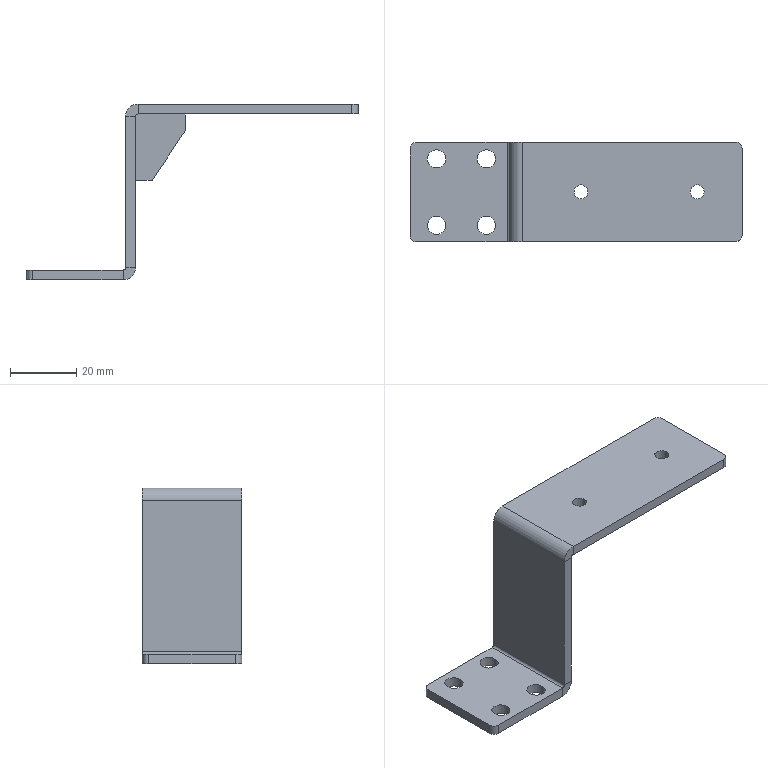Part | SolidWorks | features HoleWzd 2, Fillet 1, FlatPattern 1, ICE 1, SMBaseFlange 1, SheetMetal 1 | 1 solid | 44 faces | box 100 x 30 x 53 mm | volume 13622 mm3 | plane 23 | cylinder 21 | commonest cylinder face diameters 5.5 x8 4 x4 4.2 x4 1.5 x3 7.5 x2
STEP:
#1=CARTESIAN_POINT('',(-94.75,25.,-53.));
#2=VERTEX_POINT('',#1);
#3=CARTESIAN_POINT('',(-89.25,25.,-53.));
#4=VERTEX_POINT('',#3);
#5=CARTESIAN_POINT('',(-92.,25.,-53.));
#6=DIRECTION('',(0.,0.,1.));
#7=DIRECTION('',(1.,0.,0.));
#8=AXIS2_PLACEMENT_3D('',#5,#6,#7);
#9=CIRCLE('',#8,2.75);
#10=EDGE_CURVE('',#2,#4,#9,.T.);
#11=ORIENTED_EDGE('',*,*,#10,.F.);
#12=CARTESIAN_POINT('',(-94.75,25.,-50.));
#13=VERTEX_POINT('',#12);
#14=CARTESIAN_POINT('',(-94.75,25.,-50.));
#15=DIRECTION('',(0.,0.,1.));
#16=VECTOR('',#15,1000.);
#17=LINE('',#14,#16);
#18=EDGE_CURVE('',#2,#13,#17,.T.);
#19=ORIENTED_EDGE('',*,*,#18,.T.);
#20=CARTESIAN_POINT('',(-89.25,25.,-50.));
#21=VERTEX_POINT('',#20);
#22=CARTESIAN_POINT('',(-92.,25.,-50.));
#23=DIRECTION('',(0.,0.,1.));
#24=DIRECTION('',(1.,0.,0.));
#25=AXIS2_PLACEMENT_3D('',#22,#23,#24);
#26=CIRCLE('',#25,2.75);
#27=EDGE_CURVE('',#13,#21,#26,.T.);
#28=ORIENTED_EDGE('',*,*,#27,.T.);
#29=CARTESIAN_POINT('',(-89.25,25.,-50.));
#30=DIRECTION('',(0.,0.,1.));
#31=VECTOR('',#30,1000.);
#32=LINE('',#29,#31);
#33=EDGE_CURVE('',#4,#21,#32,.T.);
#34=ORIENTED_EDGE('',*,*,#33,.F.);
#35=EDGE_LOOP('',(#11,#19,#28,#34));
#36=FACE_OUTER_BOUND('',#35,.T.);
#37=CARTESIAN_POINT('',(-92.,25.,-50.));
#38=DIRECTION('',(0.,0.,1.));
#39=DIRECTION('',(1.,0.,0.));
#40=AXIS2_PLACEMENT_3D('',#37,#38,#39);
#41=CYLINDRICAL_SURFACE('',#40,2.75);
#42=ADVANCED_FACE('',(#36),#41,.F.);
#43=CARTESIAN_POINT('',(-79.75,25.,-53.));
#44=VERTEX_POINT('',#43);
#45=CARTESIAN_POINT('',(-74.25,25.,-53.));
#46=VERTEX_POINT('',#45);
#47=CARTESIAN_POINT('',(-77.,25.,-53.));
#48=DIRECTION('',(0.,0.,1.));
#49=DIRECTION('',(1.,0.,0.));
#50=AXIS2_PLACEMENT_3D('',#47,#48,#49);
#51=CIRCLE('',#50,2.75);
#52=EDGE_CURVE('',#44,#46,#51,.T.);
#53=ORIENTED_EDGE('',*,*,#52,.F.);
#54=CARTESIAN_POINT('',(-79.75,25.,-50.));
#55=VERTEX_POINT('',#54);
#56=CARTESIAN_POINT('',(-79.75,25.,-50.));
#57=DIRECTION('',(0.,0.,1.));
#58=VECTOR('',#57,1000.);
#59=LINE('',#56,#58);
#60=EDGE_CURVE('',#44,#55,#59,.T.);
#61=ORIENTED_EDGE('',*,*,#60,.T.);
#62=CARTESIAN_POINT('',(-74.25,25.,-50.));
#63=VERTEX_POINT('',#62);
#64=CARTESIAN_POINT('',(-77.,25.,-50.));
#65=DIRECTION('',(0.,0.,1.));
#66=DIRECTION('',(1.,0.,0.));
#67=AXIS2_PLACEMENT_3D('',#64,#65,#66);
#68=CIRCLE('',#67,2.75);
#69=EDGE_CURVE('',#55,#63,#68,.T.);
#70=ORIENTED_EDGE('',*,*,#69,.T.);
#71=CARTESIAN_POINT('',(-74.25,25.,-50.));
#72=DIRECTION('',(0.,0.,1.));
#73=VECTOR('',#72,1000.);
#74=LINE('',#71,#73);
#75=EDGE_CURVE('',#46,#63,#74,.T.);
#76=ORIENTED_EDGE('',*,*,#75,.F.);
#77=EDGE_LOOP('',(#53,#61,#70,#76));
#78=FACE_OUTER_BOUND('',#77,.T.);
#79=CARTESIAN_POINT('',(-77.,25.,-50.));
#80=DIRECTION('',(0.,0.,1.));
#81=DIRECTION('',(1.,0.,0.));
#82=AXIS2_PLACEMENT_3D('',#79,#80,#81);
#83=CYLINDRICAL_SURFACE('',#82,2.75);
#84=ADVANCED_FACE('',(#78),#83,.F.);
#85=CARTESIAN_POINT('',(-94.75,5.,-53.));
#86=VERTEX_POINT('',#85);
#87=CARTESIAN_POINT('',(-89.25,5.,-53.));
#88=VERTEX_POINT('',#87);
#89=CARTESIAN_POINT('',(-92.,5.,-53.));
#90=DIRECTION('',(0.,0.,1.));
#91=DIRECTION('',(1.,0.,0.));
#92=AXIS2_PLACEMENT_3D('',#89,#90,#91);
#93=CIRCLE('',#92,2.75);
#94=EDGE_CURVE('',#86,#88,#93,.T.);
#95=ORIENTED_EDGE('',*,*,#94,.F.);
#96=CARTESIAN_POINT('',(-94.75,5.,-50.));
#97=VERTEX_POINT('',#96);
#98=CARTESIAN_POINT('',(-94.75,5.,-50.));
#99=DIRECTION('',(0.,0.,1.));
#100=VECTOR('',#99,1000.);
#101=LINE('',#98,#100);
#102=EDGE_CURVE('',#86,#97,#101,.T.);
#103=ORIENTED_EDGE('',*,*,#102,.T.);
#104=CARTESIAN_POINT('',(-89.25,5.,-50.));
#105=VERTEX_POINT('',#104);
#106=CARTESIAN_POINT('',(-92.,5.,-50.));
#107=DIRECTION('',(0.,0.,1.));
#108=DIRECTION('',(1.,0.,0.));
#109=AXIS2_PLACEMENT_3D('',#106,#107,#108);
#110=CIRCLE('',#109,2.75);
#111=EDGE_CURVE('',#97,#105,#110,.T.);
#112=ORIENTED_EDGE('',*,*,#111,.T.);
#113=CARTESIAN_POINT('',(-89.25,5.,-50.));
#114=DIRECTION('',(0.,0.,1.));
#115=VECTOR('',#114,1000.);
#116=LINE('',#113,#115);
#117=EDGE_CURVE('',#88,#105,#116,.T.);
#118=ORIENTED_EDGE('',*,*,#117,.F.);
#119=EDGE_LOOP('',(#95,#103,#112,#118));
#120=FACE_OUTER_BOUND('',#119,.T.);
#121=CARTESIAN_POINT('',(-92.,5.,-50.));
#122=DIRECTION('',(0.,0.,1.));
#123=DIRECTION('',(1.,0.,0.));
#124=AXIS2_PLACEMENT_3D('',#121,#122,#123);
#125=CYLINDRICAL_SURFACE('',#124,2.75);
#126=ADVANCED_FACE('',(#120),#125,.F.);
#127=CARTESIAN_POINT('',(-79.75,5.,-53.));
#128=VERTEX_POINT('',#127);
#129=CARTESIAN_POINT('',(-74.25,5.,-53.));
#130=VERTEX_POINT('',#129);
#131=CARTESIAN_POINT('',(-77.,5.,-53.));
#132=DIRECTION('',(0.,0.,1.));
#133=DIRECTION('',(1.,0.,0.));
#134=AXIS2_PLACEMENT_3D('',#131,#132,#133);
#135=CIRCLE('',#134,2.75);
#136=EDGE_CURVE('',#128,#130,#135,.T.);
#137=ORIENTED_EDGE('',*,*,#136,.F.);
#138=CARTESIAN_POINT('',(-79.75,5.,-50.));
#139=VERTEX_POINT('',#138);
#140=CARTESIAN_POINT('',(-79.75,5.,-50.));
#141=DIRECTION('',(0.,0.,1.));
#142=VECTOR('',#141,1000.);
#143=LINE('',#140,#142);
#144=EDGE_CURVE('',#128,#139,#143,.T.);
#145=ORIENTED_EDGE('',*,*,#144,.T.);
#146=CARTESIAN_POINT('',(-74.25,5.,-50.));
#147=VERTEX_POINT('',#146);
#148=CARTESIAN_POINT('',(-77.,5.,-50.));
#149=DIRECTION('',(0.,0.,1.));
#150=DIRECTION('',(1.,0.,0.));
#151=AXIS2_PLACEMENT_3D('',#148,#149,#150);
#152=CIRCLE('',#151,2.75);
#153=EDGE_CURVE('',#139,#147,#152,.T.);
#154=ORIENTED_EDGE('',*,*,#153,.T.);
#155=CARTESIAN_POINT('',(-74.25,5.,-50.));
#156=DIRECTION('',(0.,0.,1.));
#157=VECTOR('',#156,1000.);
#158=LINE('',#155,#157);
#159=EDGE_CURVE('',#130,#147,#158,.T.);
#160=ORIENTED_EDGE('',*,*,#159,.F.);
#161=EDGE_LOOP('',(#137,#145,#154,#160));
#162=FACE_OUTER_BOUND('',#161,.T.);
#163=CARTESIAN_POINT('',(-77.,5.,-50.));
#164=DIRECTION('',(0.,0.,1.));
#165=DIRECTION('',(1.,0.,0.));
#166=AXIS2_PLACEMENT_3D('',#163,#164,#165);
#167=CYLINDRICAL_SURFACE('',#166,2.75);
#168=ADVANCED_FACE('',(#162),#167,.F.);
#169=CARTESIAN_POINT('',(-50.6,14.997,-3.));
#170=VERTEX_POINT('',#169);
#171=CARTESIAN_POINT('',(-46.4,14.997,-3.));
#172=VERTEX_POINT('',#171);
#173=CARTESIAN_POINT('',(-48.5,14.997,-3.));
#174=DIRECTION('',(0.,0.,1.));
#175=DIRECTION('',(1.,0.,0.));
#176=AXIS2_PLACEMENT_3D('',#173,#174,#175);
#177=CIRCLE('',#176,2.1);
#178=EDGE_CURVE('',#170,#172,#177,.T.);
#179=ORIENTED_EDGE('',*,*,#178,.F.);
#180=CARTESIAN_POINT('',(-50.6,14.997,0.));
#181=VERTEX_POINT('',#180);
#182=CARTESIAN_POINT('',(-50.6,14.997,0.));
#183=DIRECTION('',(0.,0.,1.));
#184=VECTOR('',#183,1000.);
#185=LINE('',#182,#184);
#186=EDGE_CURVE('',#170,#181,#185,.T.);
#187=ORIENTED_EDGE('',*,*,#186,.T.);
#188=CARTESIAN_POINT('',(-46.4,14.997,0.));
#189=VERTEX_POINT('',#188);
#190=CARTESIAN_POINT('',(-48.5,14.997,0.));
#191=DIRECTION('',(0.,0.,1.));
#192=DIRECTION('',(1.,0.,0.));
#193=AXIS2_PLACEMENT_3D('',#190,#191,#192);
#194=CIRCLE('',#193,2.1);
#195=EDGE_CURVE('',#181,#189,#194,.T.);
#196=ORIENTED_EDGE('',*,*,#195,.T.);
#197=CARTESIAN_POINT('',(-46.4,14.997,0.));
#198=DIRECTION('',(0.,0.,1.));
#199=VECTOR('',#198,1000.);
#200=LINE('',#197,#199);
#201=EDGE_CURVE('',#172,#189,#200,.T.);
#202=ORIENTED_EDGE('',*,*,#201,.F.);
#203=EDGE_LOOP('',(#179,#187,#196,#202));
#204=FACE_OUTER_BOUND('',#203,.T.);
#205=CARTESIAN_POINT('',(-48.5,14.997,0.));
#206=DIRECTION('',(0.,0.,1.));
#207=DIRECTION('',(1.,0.,0.));
#208=AXIS2_PLACEMENT_3D('',#205,#206,#207);
#209=CYLINDRICAL_SURFACE('',#208,2.1);
#210=ADVANCED_FACE('',(#204),#209,.F.);
#211=CARTESIAN_POINT('',(-15.6,14.997,-3.));
#212=VERTEX_POINT('',#211);
#213=CARTESIAN_POINT('',(-11.4,14.997,-3.));
#214=VERTEX_POINT('',#213);
#215=CARTESIAN_POINT('',(-13.5,14.997,-3.));
#216=DIRECTION('',(0.,0.,1.));
#217=DIRECTION('',(1.,0.,0.));
#218=AXIS2_PLACEMENT_3D('',#215,#216,#217);
#219=CIRCLE('',#218,2.1);
#220=EDGE_CURVE('',#212,#214,#219,.T.);
#221=ORIENTED_EDGE('',*,*,#220,.F.);
#222=CARTESIAN_POINT('',(-15.6,14.997,0.));
#223=VERTEX_POINT('',#222);
#224=CARTESIAN_POINT('',(-15.6,14.997,0.));
#225=DIRECTION('',(0.,0.,1.));
#226=VECTOR('',#225,1000.);
#227=LINE('',#224,#226);
#228=EDGE_CURVE('',#212,#223,#227,.T.);
#229=ORIENTED_EDGE('',*,*,#228,.T.);
#230=CARTESIAN_POINT('',(-11.4,14.997,0.));
#231=VERTEX_POINT('',#230);
#232=CARTESIAN_POINT('',(-13.5,14.997,0.));
#233=DIRECTION('',(0.,0.,1.));
#234=DIRECTION('',(1.,0.,0.));
#235=AXIS2_PLACEMENT_3D('',#232,#233,#234);
#236=CIRCLE('',#235,2.1);
#237=EDGE_CURVE('',#223,#231,#236,.T.);
#238=ORIENTED_EDGE('',*,*,#237,.T.);
#239=CARTESIAN_POINT('',(-11.4,14.997,0.));
#240=DIRECTION('',(0.,0.,1.));
#241=VECTOR('',#240,1000.);
#242=LINE('',#239,#241);
#243=EDGE_CURVE('',#214,#231,#242,.T.);
#244=ORIENTED_EDGE('',*,*,#243,.F.);
#245=EDGE_LOOP('',(#221,#229,#238,#244));
#246=FACE_OUTER_BOUND('',#245,.T.);
#247=CARTESIAN_POINT('',(-13.5,14.997,0.));
#248=DIRECTION('',(0.,0.,1.));
#249=DIRECTION('',(1.,0.,0.));
#250=AXIS2_PLACEMENT_3D('',#247,#248,#249);
#251=CYLINDRICAL_SURFACE('',#250,2.1);
#252=ADVANCED_FACE('',(#246),#251,.F.);
#253=CARTESIAN_POINT('',(-67.,13.5,-3.75));
#254=VERTEX_POINT('',#253);
#255=CARTESIAN_POINT('',(-66.25,13.5,-3.));
#256=VERTEX_POINT('',#255);
#257=CARTESIAN_POINT('',(-66.25,13.5,-3.75));
#258=DIRECTION('',(0.,1.,0.));
#259=DIRECTION('',(0.,0.,1.));
#260=AXIS2_PLACEMENT_3D('',#257,#258,#259);
#261=CIRCLE('',#260,0.75);
#262=EDGE_CURVE('',#254,#256,#261,.T.);
#263=ORIENTED_EDGE('',*,*,#262,.T.);
#264=CARTESIAN_POINT('',(-66.25,0.,-3.));
#265=VERTEX_POINT('',#264);
#266=CARTESIAN_POINT('',(-66.25,30.,-3.));
#267=DIRECTION('',(0.,-1.,0.));
#268=VECTOR('',#267,1000.);
#269=LINE('',#266,#268);
#270=EDGE_CURVE('',#256,#265,#269,.T.);
#271=ORIENTED_EDGE('',*,*,#270,.T.);
#272=CARTESIAN_POINT('',(-67.,0.,-3.75));
#273=VERTEX_POINT('',#272);
#274=CARTESIAN_POINT('',(-66.25,0.,-3.75));
#275=DIRECTION('',(0.,-1.,0.));
#276=DIRECTION('',(1.,0.,0.));
#277=AXIS2_PLACEMENT_3D('',#274,#275,#276);
#278=CIRCLE('',#277,0.75);
#279=EDGE_CURVE('',#265,#273,#278,.T.);
#280=ORIENTED_EDGE('',*,*,#279,.T.);
#281=CARTESIAN_POINT('',(-67.,30.,-3.75));
#282=DIRECTION('',(0.,-1.,0.));
#283=VECTOR('',#282,1000.);
#284=LINE('',#281,#283);
#285=EDGE_CURVE('',#254,#273,#284,.T.);
#286=ORIENTED_EDGE('',*,*,#285,.F.);
#287=EDGE_LOOP('',(#263,#271,#280,#286));
#288=FACE_OUTER_BOUND('',#287,.T.);
#289=CARTESIAN_POINT('',(-66.25,30.,-3.75));
#290=DIRECTION('',(0.,-1.,0.));
#291=DIRECTION('',(0.,0.,-1.));
#292=AXIS2_PLACEMENT_3D('',#289,#290,#291);
#293=CYLINDRICAL_SURFACE('',#292,0.75);
#294=ADVANCED_FACE('',(#288),#293,.F.);
#295=CARTESIAN_POINT('',(-70.,30.,-3.75));
#296=VERTEX_POINT('',#295);
#297=CARTESIAN_POINT('',(-67.,30.,-3.75));
#298=VERTEX_POINT('',#297);
#299=CARTESIAN_POINT('',(-70.,30.,-3.75));
#300=DIRECTION('',(1.,0.,0.));
#301=VECTOR('',#300,1000.);
#302=LINE('',#299,#301);
#303=EDGE_CURVE('',#296,#298,#302,.T.);
#304=ORIENTED_EDGE('',*,*,#303,.F.);
#305=CARTESIAN_POINT('',(-66.25,30.,0.));
#306=VERTEX_POINT('',#305);
#307=CARTESIAN_POINT('',(-66.25,30.,-3.75));
#308=DIRECTION('',(0.,-1.,0.));
#309=DIRECTION('',(0.,0.,1.));
#310=AXIS2_PLACEMENT_3D('',#307,#308,#309);
#311=CIRCLE('',#310,3.75);
#312=EDGE_CURVE('',#306,#296,#311,.T.);
#313=ORIENTED_EDGE('',*,*,#312,.F.);
#314=CARTESIAN_POINT('',(-66.25,30.,-3.));
#315=VERTEX_POINT('',#314);
#316=CARTESIAN_POINT('',(-66.25,30.,-3.));
#317=DIRECTION('',(0.,0.,1.));
#318=VECTOR('',#317,1000.);
#319=LINE('',#316,#318);
#320=EDGE_CURVE('',#315,#306,#319,.T.);
#321=ORIENTED_EDGE('',*,*,#320,.F.);
#322=CARTESIAN_POINT('',(-66.25,30.,-3.75));
#323=DIRECTION('',(0.,-1.,0.));
#324=DIRECTION('',(1.,0.,0.));
#325=AXIS2_PLACEMENT_3D('',#322,#323,#324);
#326=CIRCLE('',#325,0.75);
#327=EDGE_CURVE('',#315,#298,#326,.T.);
#328=ORIENTED_EDGE('',*,*,#327,.T.);
#329=EDGE_LOOP('',(#304,#313,#321,#328));
#330=FACE_OUTER_BOUND('',#329,.T.);
#331=CARTESIAN_POINT('',(-70.,30.,-3.75));
#332=DIRECTION('',(0.,1.,0.));
#333=DIRECTION('',(0.,0.,1.));
#334=AXIS2_PLACEMENT_3D('',#331,#332,#333);
#335=PLANE('',#334);
#336=ADVANCED_FACE('',(#330),#335,.T.);
#337=CARTESIAN_POINT('',(-70.,30.,-49.25));
#338=VERTEX_POINT('',#337);
#339=CARTESIAN_POINT('',(-70.,30.,0.));
#340=DIRECTION('',(0.,0.,-1.));
#341=VECTOR('',#340,1000.);
#342=LINE('',#339,#341);
#343=EDGE_CURVE('',#296,#338,#342,.T.);
#344=ORIENTED_EDGE('',*,*,#343,.F.);
#345=ORIENTED_EDGE('',*,*,#303,.T.);
#346=CARTESIAN_POINT('',(-67.,30.,-49.25));
#347=VERTEX_POINT('',#346);
#348=CARTESIAN_POINT('',(-67.,30.,0.));
#349=DIRECTION('',(0.,0.,-1.));
#350=VECTOR('',#349,1000.);
#351=LINE('',#348,#350);
#352=EDGE_CURVE('',#298,#347,#351,.T.);
#353=ORIENTED_EDGE('',*,*,#352,.T.);
#354=CARTESIAN_POINT('',(-67.,30.,-49.25));
#355=DIRECTION('',(-1.,0.,0.));
#356=VECTOR('',#355,1000.);
#357=LINE('',#354,#356);
#358=EDGE_CURVE('',#347,#338,#357,.T.);
#359=ORIENTED_EDGE('',*,*,#358,.T.);
#360=EDGE_LOOP('',(#344,#345,#353,#359));
#361=FACE_OUTER_BOUND('',#360,.T.);
#362=CARTESIAN_POINT('',(-66.25,30.,-3.));
#363=DIRECTION('',(0.,1.,0.));
#364=DIRECTION('',(0.,0.,1.));
#365=AXIS2_PLACEMENT_3D('',#362,#363,#364);
#366=PLANE('',#365);
#367=ADVANCED_FACE('',(#361),#366,.T.);
#368=CARTESIAN_POINT('',(-66.25,0.,0.));
#369=VERTEX_POINT('',#368);
#370=CARTESIAN_POINT('',(-66.25,0.,0.));
#371=DIRECTION('',(0.,0.,-1.));
#372=VECTOR('',#371,1000.);
#373=LINE('',#370,#372);
#374=EDGE_CURVE('',#369,#265,#373,.T.);
#375=ORIENTED_EDGE('',*,*,#374,.F.);
#376=CARTESIAN_POINT('',(-70.,0.,-3.75));
#377=VERTEX_POINT('',#376);
#378=CARTESIAN_POINT('',(-66.25,0.,-3.75));
#379=DIRECTION('',(0.,-1.,0.));
#380=DIRECTION('',(0.,0.,1.));
#381=AXIS2_PLACEMENT_3D('',#378,#379,#380);
#382=CIRCLE('',#381,3.75);
#383=EDGE_CURVE('',#369,#377,#382,.T.);
#384=ORIENTED_EDGE('',*,*,#383,.T.);
#385=CARTESIAN_POINT('',(-67.,0.,-3.75));
#386=DIRECTION('',(-1.,0.,0.));
#387=VECTOR('',#386,1000.);
#388=LINE('',#385,#387);
#389=EDGE_CURVE('',#273,#377,#388,.T.);
#390=ORIENTED_EDGE('',*,*,#389,.F.);
#391=ORIENTED_EDGE('',*,*,#279,.F.);
#392=EDGE_LOOP('',(#375,#384,#390,#391));
#393=FACE_OUTER_BOUND('',#392,.T.);
#394=CARTESIAN_POINT('',(-66.25,0.,0.));
#395=DIRECTION('',(0.,-1.,0.));
#396=DIRECTION('',(0.,0.,-1.));
#397=AXIS2_PLACEMENT_3D('',#394,#395,#396);
#398=PLANE('',#397);
#399=ADVANCED_FACE('',(#393),#398,.T.);
#400=CARTESIAN_POINT('',(-2.,0.,-3.));
#401=VERTEX_POINT('',#400);
#402=CARTESIAN_POINT('',(0.,0.,-3.));
#403=DIRECTION('',(-1.,0.,0.));
#404=VECTOR('',#403,1000.);
#405=LINE('',#402,#404);
#406=EDGE_CURVE('',#401,#265,#405,.T.);
#407=ORIENTED_EDGE('',*,*,#406,.F.);
#408=CARTESIAN_POINT('',(-2.,0.,0.));
#409=VERTEX_POINT('',#408);
#410=CARTESIAN_POINT('',(-2.,0.,-3.75));
#411=DIRECTION('',(0.,0.,1.));
#412=VECTOR('',#411,1000.);
#413=LINE('',#410,#412);
#414=EDGE_CURVE('',#401,#409,#413,.T.);
#415=ORIENTED_EDGE('',*,*,#414,.T.);
#416=CARTESIAN_POINT('',(0.,0.,0.));
#417=DIRECTION('',(-1.,0.,0.));
#418=VECTOR('',#417,1000.);
#419=LINE('',#416,#418);
#420=EDGE_CURVE('',#409,#369,#419,.T.);
#421=ORIENTED_EDGE('',*,*,#420,.T.);
#422=ORIENTED_EDGE('',*,*,#374,.T.);
#423=EDGE_LOOP('',(#407,#415,#421,#422));
#424=FACE_OUTER_BOUND('',#423,.T.);
#425=CARTESIAN_POINT('',(-67.,0.,-3.75));
#426=DIRECTION('',(0.,-1.,0.));
#427=DIRECTION('',(0.,0.,-1.));
#428=AXIS2_PLACEMENT_3D('',#425,#426,#427);
#429=PLANE('',#428);
#430=ADVANCED_FACE('',(#424),#429,.T.);
#431=CARTESIAN_POINT('',(-70.75,30.,-50.));
#432=VERTEX_POINT('',#431);
#433=CARTESIAN_POINT('',(-70.75,30.,-53.));
#434=VERTEX_POINT('',#433);
#435=CARTESIAN_POINT('',(-70.75,30.,-50.));
#436=DIRECTION('',(0.,0.,-1.));
#437=VECTOR('',#436,1000.);
#438=LINE('',#435,#437);
#439=EDGE_CURVE('',#432,#434,#438,.T.);
#440=ORIENTED_EDGE('',*,*,#439,.F.);
#441=CARTESIAN_POINT('',(-70.75,30.,-49.25));
#442=DIRECTION('',(0.,1.,0.));
#443=DIRECTION('',(0.,0.,-1.));
#444=AXIS2_PLACEMENT_3D('',#441,#442,#443);
#445=CIRCLE('',#444,0.75);
#446=EDGE_CURVE('',#338,#432,#445,.T.);
#447=ORIENTED_EDGE('',*,*,#446,.F.);
#448=ORIENTED_EDGE('',*,*,#358,.F.);
#449=CARTESIAN_POINT('',(-70.75,30.,-49.25));
#450=DIRECTION('',(0.,1.,0.));
#451=DIRECTION('',(1.,0.,0.));
#452=AXIS2_PLACEMENT_3D('',#449,#450,#451);
#453=CIRCLE('',#452,3.75);
#454=EDGE_CURVE('',#347,#434,#453,.T.);
#455=ORIENTED_EDGE('',*,*,#454,.T.);
#456=EDGE_LOOP('',(#440,#447,#448,#455));
#457=FACE_OUTER_BOUND('',#456,.T.);
#458=CARTESIAN_POINT('',(-70.75,30.,-50.));
#459=DIRECTION('',(0.,1.,0.));
#460=DIRECTION('',(0.,0.,1.));
#461=AXIS2_PLACEMENT_3D('',#458,#459,#460);
#462=PLANE('',#461);
#463=ADVANCED_FACE('',(#457),#462,.T.);
#464=CARTESIAN_POINT('',(-98.,30.,-53.));
#465=VERTEX_POINT('',#464);
#466=CARTESIAN_POINT('',(-70.,30.,-53.));
#467=DIRECTION('',(-1.,0.,0.));
#468=VECTOR('',#467,1000.);
#469=LINE('',#466,#468);
#470=EDGE_CURVE('',#434,#465,#469,.T.);
#471=ORIENTED_EDGE('',*,*,#470,.T.);
#472=CARTESIAN_POINT('',(-98.,30.,-50.));
#473=VERTEX_POINT('',#472);
#474=CARTESIAN_POINT('',(-98.,30.,-49.25));
#475=DIRECTION('',(0.,0.,1.));
#476=VECTOR('',#475,1000.);
#477=LINE('',#474,#476);
#478=EDGE_CURVE('',#465,#473,#477,.T.);
#479=ORIENTED_EDGE('',*,*,#478,.T.);
#480=CARTESIAN_POINT('',(-70.,30.,-50.));
#481=DIRECTION('',(-1.,0.,0.));
#482=VECTOR('',#481,1000.);
#483=LINE('',#480,#482);
#484=EDGE_CURVE('',#432,#473,#483,.T.);
#485=ORIENTED_EDGE('',*,*,#484,.F.);
#486=ORIENTED_EDGE('',*,*,#439,.T.);
#487=EDGE_LOOP('',(#471,#479,#485,#486));
#488=FACE_OUTER_BOUND('',#487,.T.);
#489=CARTESIAN_POINT('',(-67.,30.,-49.25));
#490=DIRECTION('',(0.,1.,0.));
#491=DIRECTION('',(0.,0.,1.));
#492=AXIS2_PLACEMENT_3D('',#489,#490,#491);
#493=PLANE('',#492);
#494=ADVANCED_FACE('',(#488),#493,.T.);
#495=CARTESIAN_POINT('',(-70.,0.,-49.25));
#496=VERTEX_POINT('',#495);
#497=CARTESIAN_POINT('',(-67.,0.,-49.25));
#498=VERTEX_POINT('',#497);
#499=CARTESIAN_POINT('',(-70.,0.,-49.25));
#500=DIRECTION('',(1.,0.,0.));
#501=VECTOR('',#500,1000.);
#502=LINE('',#499,#501);
#503=EDGE_CURVE('',#496,#498,#502,.T.);
#504=ORIENTED_EDGE('',*,*,#503,.F.);
#505=CARTESIAN_POINT('',(-70.75,0.,-50.));
#506=VERTEX_POINT('',#505);
#507=CARTESIAN_POINT('',(-70.75,0.,-49.25));
#508=DIRECTION('',(0.,1.,0.));
#509=DIRECTION('',(0.,0.,-1.));
#510=AXIS2_PLACEMENT_3D('',#507,#508,#509);
#511=CIRCLE('',#510,0.75);
#512=EDGE_CURVE('',#496,#506,#511,.T.);
#513=ORIENTED_EDGE('',*,*,#512,.T.);
#514=CARTESIAN_POINT('',(-70.75,0.,-53.));
#515=VERTEX_POINT('',#514);
#516=CARTESIAN_POINT('',(-70.75,0.,-53.));
#517=DIRECTION('',(0.,0.,1.));
#518=VECTOR('',#517,1000.);
#519=LINE('',#516,#518);
#520=EDGE_CURVE('',#515,#506,#519,.T.);
#521=ORIENTED_EDGE('',*,*,#520,.F.);
#522=CARTESIAN_POINT('',(-70.75,0.,-49.25));
#523=DIRECTION('',(0.,1.,0.));
#524=DIRECTION('',(1.,0.,0.));
#525=AXIS2_PLACEMENT_3D('',#522,#523,#524);
#526=CIRCLE('',#525,3.75);
#527=EDGE_CURVE('',#498,#515,#526,.T.);
#528=ORIENTED_EDGE('',*,*,#527,.F.);
#529=EDGE_LOOP('',(#504,#513,#521,#528));
#530=FACE_OUTER_BOUND('',#529,.T.);
#531=CARTESIAN_POINT('',(-70.,0.,-49.25));
#532=DIRECTION('',(0.,-1.,0.));
#533=DIRECTION('',(0.,0.,-1.));
#534=AXIS2_PLACEMENT_3D('',#531,#532,#533);
#535=PLANE('',#534);
#536=ADVANCED_FACE('',(#530),#535,.T.);
#537=CARTESIAN_POINT('',(-70.,0.,0.));
#538=DIRECTION('',(0.,0.,-1.));
#539=VECTOR('',#538,1000.);
#540=LINE('',#537,#539);
#541=EDGE_CURVE('',#377,#496,#540,.T.);
#542=ORIENTED_EDGE('',*,*,#541,.T.);
#543=ORIENTED_EDGE('',*,*,#503,.T.);
#544=CARTESIAN_POINT('',(-67.,0.,0.));
#545=DIRECTION('',(0.,0.,-1.));
#546=VECTOR('',#545,1000.);
#547=LINE('',#544,#546);
#548=EDGE_CURVE('',#273,#498,#547,.T.);
#549=ORIENTED_EDGE('',*,*,#548,.F.);
#550=ORIENTED_EDGE('',*,*,#389,.T.);
#551=EDGE_LOOP('',(#542,#543,#549,#550));
#552=FACE_OUTER_BOUND('',#551,.T.);
#553=CARTESIAN_POINT('',(-70.75,0.,-53.));
#554=DIRECTION('',(0.,-1.,0.));
#555=DIRECTION('',(0.,0.,-1.));
#556=AXIS2_PLACEMENT_3D('',#553,#554,#555);
#557=PLANE('',#556);
#558=ADVANCED_FACE('',(#552),#557,.T.);
#559=CARTESIAN_POINT('',(-92.,25.,-53.));
#560=DIRECTION('',(0.,0.,1.));
#561=DIRECTION('',(1.,0.,0.));
#562=AXIS2_PLACEMENT_3D('',#559,#560,#561);
#563=CIRCLE('',#562,2.75);
#564=EDGE_CURVE('',#4,#2,#563,.T.);
#565=ORIENTED_EDGE('',*,*,#564,.T.);
#566=ORIENTED_EDGE('',*,*,#10,.T.);
#567=EDGE_LOOP('',(#565,#566));
#568=FACE_BOUND('',#567,.T.);
#569=CARTESIAN_POINT('',(-77.,25.,-53.));
#570=DIRECTION('',(0.,0.,1.));
#571=DIRECTION('',(1.,0.,0.));
#572=AXIS2_PLACEMENT_3D('',#569,#570,#571);
#573=CIRCLE('',#572,2.75);
#574=EDGE_CURVE('',#46,#44,#573,.T.);
#575=ORIENTED_EDGE('',*,*,#574,.T.);
#576=ORIENTED_EDGE('',*,*,#52,.T.);
#577=EDGE_LOOP('',(#575,#576));
#578=FACE_BOUND('',#577,.T.);
#579=CARTESIAN_POINT('',(-92.,5.,-53.));
#580=DIRECTION('',(0.,0.,1.));
#581=DIRECTION('',(1.,0.,0.));
#582=AXIS2_PLACEMENT_3D('',#579,#580,#581);
#583=CIRCLE('',#582,2.75);
#584=EDGE_CURVE('',#88,#86,#583,.T.);
#585=ORIENTED_EDGE('',*,*,#584,.T.);
#586=ORIENTED_EDGE('',*,*,#94,.T.);
#587=EDGE_LOOP('',(#585,#586));
#588=FACE_BOUND('',#587,.T.);
#589=CARTESIAN_POINT('',(-77.,5.,-53.));
#590=DIRECTION('',(0.,0.,1.));
#591=DIRECTION('',(1.,0.,0.));
#592=AXIS2_PLACEMENT_3D('',#589,#590,#591);
#593=CIRCLE('',#592,2.75);
#594=EDGE_CURVE('',#130,#128,#593,.T.);
#595=ORIENTED_EDGE('',*,*,#594,.T.);
#596=ORIENTED_EDGE('',*,*,#136,.T.);
#597=EDGE_LOOP('',(#595,#596));
#598=FACE_BOUND('',#597,.T.);
#599=CARTESIAN_POINT('',(-98.,0.,-53.));
#600=VERTEX_POINT('',#599);
#601=CARTESIAN_POINT('',(-70.,0.,-53.));
#602=DIRECTION('',(-1.,0.,0.));
#603=VECTOR('',#602,1000.);
#604=LINE('',#601,#603);
#605=EDGE_CURVE('',#515,#600,#604,.T.);
#606=ORIENTED_EDGE('',*,*,#605,.T.);
#607=CARTESIAN_POINT('',(-100.,2.,-53.));
#608=VERTEX_POINT('',#607);
#609=CARTESIAN_POINT('',(-98.,2.,-53.));
#610=DIRECTION('',(0.,0.,-1.));
#611=DIRECTION('',(1.,0.,0.));
#612=AXIS2_PLACEMENT_3D('',#609,#610,#611);
#613=CIRCLE('',#612,2.);
#614=EDGE_CURVE('',#600,#608,#613,.T.);
#615=ORIENTED_EDGE('',*,*,#614,.T.);
#616=CARTESIAN_POINT('',(-100.,28.,-53.));
#617=VERTEX_POINT('',#616);
#618=CARTESIAN_POINT('',(-100.,30.,-53.));
#619=DIRECTION('',(0.,-1.,0.));
#620=VECTOR('',#619,1000.);
#621=LINE('',#618,#620);
#622=EDGE_CURVE('',#617,#608,#621,.T.);
#623=ORIENTED_EDGE('',*,*,#622,.F.);
#624=CARTESIAN_POINT('',(-98.,28.,-53.));
#625=DIRECTION('',(0.,0.,-1.));
#626=DIRECTION('',(1.,0.,0.));
#627=AXIS2_PLACEMENT_3D('',#624,#625,#626);
#628=CIRCLE('',#627,2.);
#629=EDGE_CURVE('',#617,#465,#628,.T.);
#630=ORIENTED_EDGE('',*,*,#629,.T.);
#631=ORIENTED_EDGE('',*,*,#470,.F.);
#632=CARTESIAN_POINT('',(-70.75,30.,-53.));
#633=DIRECTION('',(0.,-1.,0.));
#634=VECTOR('',#633,1000.);
#635=LINE('',#632,#634);
#636=EDGE_CURVE('',#434,#515,#635,.T.);
#637=ORIENTED_EDGE('',*,*,#636,.T.);
#638=EDGE_LOOP('',(#606,#615,#623,#630,#631,#637));
#639=FACE_OUTER_BOUND('',#638,.T.);
#640=CARTESIAN_POINT('',(-70.,30.,-53.));
#641=DIRECTION('',(0.,0.,1.));
#642=DIRECTION('',(1.,0.,0.));
#643=AXIS2_PLACEMENT_3D('',#640,#641,#642);
#644=PLANE('',#643);
#645=ADVANCED_FACE('',(#568,#578,#588,#598,#639),#644,.F.);
#646=ORIENTED_EDGE('',*,*,#622,.T.);
#647=CARTESIAN_POINT('',(-100.,2.,-50.));
#648=VERTEX_POINT('',#647);
#649=CARTESIAN_POINT('',(-100.,2.,-50.));
#650=DIRECTION('',(0.,0.,1.));
#651=VECTOR('',#650,1000.);
#652=LINE('',#649,#651);
#653=EDGE_CURVE('',#608,#648,#652,.T.);
#654=ORIENTED_EDGE('',*,*,#653,.T.);
#655=CARTESIAN_POINT('',(-100.,28.,-50.));
#656=VERTEX_POINT('',#655);
#657=CARTESIAN_POINT('',(-100.,30.,-50.));
#658=DIRECTION('',(0.,-1.,0.));
#659=VECTOR('',#658,1000.);
#660=LINE('',#657,#659);
#661=EDGE_CURVE('',#656,#648,#660,.T.);
#662=ORIENTED_EDGE('',*,*,#661,.F.);
#663=CARTESIAN_POINT('',(-100.,28.,-50.));
#664=DIRECTION('',(0.,0.,-1.));
#665=VECTOR('',#664,1000.);
#666=LINE('',#663,#665);
#667=EDGE_CURVE('',#656,#617,#666,.T.);
#668=ORIENTED_EDGE('',*,*,#667,.T.);
#669=EDGE_LOOP('',(#646,#654,#662,#668));
#670=FACE_OUTER_BOUND('',#669,.T.);
#671=CARTESIAN_POINT('',(-100.,30.,-50.));
#672=DIRECTION('',(-1.,0.,0.));
#673=DIRECTION('',(0.,0.,1.));
#674=AXIS2_PLACEMENT_3D('',#671,#672,#673);
#675=PLANE('',#674);
#676=ADVANCED_FACE('',(#670),#675,.T.);
#677=CARTESIAN_POINT('',(-92.,25.,-50.));
#678=DIRECTION('',(0.,0.,1.));
#679=DIRECTION('',(1.,0.,0.));
#680=AXIS2_PLACEMENT_3D('',#677,#678,#679);
#681=CIRCLE('',#680,2.75);
#682=EDGE_CURVE('',#21,#13,#681,.T.);
#683=ORIENTED_EDGE('',*,*,#682,.F.);
#684=ORIENTED_EDGE('',*,*,#27,.F.);
#685=EDGE_LOOP('',(#683,#684));
#686=FACE_BOUND('',#685,.T.);
#687=CARTESIAN_POINT('',(-77.,25.,-50.));
#688=DIRECTION('',(0.,0.,1.));
#689=DIRECTION('',(1.,0.,0.));
#690=AXIS2_PLACEMENT_3D('',#687,#688,#689);
#691=CIRCLE('',#690,2.75);
#692=EDGE_CURVE('',#63,#55,#691,.T.);
#693=ORIENTED_EDGE('',*,*,#692,.F.);
#694=ORIENTED_EDGE('',*,*,#69,.F.);
#695=EDGE_LOOP('',(#693,#694));
#696=FACE_BOUND('',#695,.T.);
#697=CARTESIAN_POINT('',(-92.,5.,-50.));
#698=DIRECTION('',(0.,0.,1.));
#699=DIRECTION('',(1.,0.,0.));
#700=AXIS2_PLACEMENT_3D('',#697,#698,#699);
#701=CIRCLE('',#700,2.75);
#702=EDGE_CURVE('',#105,#97,#701,.T.);
#703=ORIENTED_EDGE('',*,*,#702,.F.);
#704=ORIENTED_EDGE('',*,*,#111,.F.);
#705=EDGE_LOOP('',(#703,#704));
#706=FACE_BOUND('',#705,.T.);
#707=CARTESIAN_POINT('',(-77.,5.,-50.));
#708=DIRECTION('',(0.,0.,1.));
#709=DIRECTION('',(1.,0.,0.));
#710=AXIS2_PLACEMENT_3D('',#707,#708,#709);
#711=CIRCLE('',#710,2.75);
#712=EDGE_CURVE('',#147,#139,#711,.T.);
#713=ORIENTED_EDGE('',*,*,#712,.F.);
#714=ORIENTED_EDGE('',*,*,#153,.F.);
#715=EDGE_LOOP('',(#713,#714));
#716=FACE_BOUND('',#715,.T.);
#717=ORIENTED_EDGE('',*,*,#661,.T.);
#718=CARTESIAN_POINT('',(-98.,0.,-50.));
#719=VERTEX_POINT('',#718);
#720=CARTESIAN_POINT('',(-98.,2.,-50.));
#721=DIRECTION('',(0.,0.,1.));
#722=DIRECTION('',(1.,0.,0.));
#723=AXIS2_PLACEMENT_3D('',#720,#721,#722);
#724=CIRCLE('',#723,2.);
#725=EDGE_CURVE('',#648,#719,#724,.T.);
#726=ORIENTED_EDGE('',*,*,#725,.T.);
#727=CARTESIAN_POINT('',(-70.,0.,-50.));
#728=DIRECTION('',(-1.,0.,0.));
#729=VECTOR('',#728,1000.);
#730=LINE('',#727,#729);
#731=EDGE_CURVE('',#506,#719,#730,.T.);
#732=ORIENTED_EDGE('',*,*,#731,.F.);
#733=CARTESIAN_POINT('',(-70.75,30.,-50.));
#734=DIRECTION('',(0.,-1.,0.));
#735=VECTOR('',#734,1000.);
#736=LINE('',#733,#735);
#737=EDGE_CURVE('',#432,#506,#736,.T.);
#738=ORIENTED_EDGE('',*,*,#737,.F.);
#739=ORIENTED_EDGE('',*,*,#484,.T.);
#740=CARTESIAN_POINT('',(-98.,28.,-50.));
#741=DIRECTION('',(0.,0.,1.));
#742=DIRECTION('',(1.,0.,0.));
#743=AXIS2_PLACEMENT_3D('',#740,#741,#742);
#744=CIRCLE('',#743,2.);
#745=EDGE_CURVE('',#473,#656,#744,.T.);
#746=ORIENTED_EDGE('',*,*,#745,.T.);
#747=EDGE_LOOP('',(#717,#726,#732,#738,#739,#746));
#748=FACE_OUTER_BOUND('',#747,.T.);
#749=CARTESIAN_POINT('',(-70.,30.,-50.));
#750=DIRECTION('',(0.,0.,1.));
#751=DIRECTION('',(1.,0.,0.));
#752=AXIS2_PLACEMENT_3D('',#749,#750,#751);
#753=PLANE('',#752);
#754=ADVANCED_FACE('',(#686,#696,#706,#716,#748),#753,.T.);
#755=ORIENTED_EDGE('',*,*,#512,.F.);
#756=CARTESIAN_POINT('',(-70.,30.,-49.25));
#757=DIRECTION('',(0.,-1.,0.));
#758=VECTOR('',#757,1000.);
#759=LINE('',#756,#758);
#760=EDGE_CURVE('',#338,#496,#759,.T.);
#761=ORIENTED_EDGE('',*,*,#760,.F.);
#762=ORIENTED_EDGE('',*,*,#446,.T.);
#763=ORIENTED_EDGE('',*,*,#737,.T.);
#764=EDGE_LOOP('',(#755,#761,#762,#763));
#765=FACE_OUTER_BOUND('',#764,.T.);
#766=CARTESIAN_POINT('',(-70.75,30.,-49.25));
#767=DIRECTION('',(0.,-1.,0.));
#768=DIRECTION('',(0.,0.,-1.));
#769=AXIS2_PLACEMENT_3D('',#766,#767,#768);
#770=CYLINDRICAL_SURFACE('',#769,0.75);
#771=ADVANCED_FACE('',(#765),#770,.F.);
#772=ORIENTED_EDGE('',*,*,#541,.F.);
#773=CARTESIAN_POINT('',(-70.,30.,-3.75));
#774=DIRECTION('',(0.,-1.,0.));
#775=VECTOR('',#774,1000.);
#776=LINE('',#773,#775);
#777=EDGE_CURVE('',#296,#377,#776,.T.);
#778=ORIENTED_EDGE('',*,*,#777,.F.);
#779=ORIENTED_EDGE('',*,*,#343,.T.);
#780=ORIENTED_EDGE('',*,*,#760,.T.);
#781=EDGE_LOOP('',(#772,#778,#779,#780));
#782=FACE_OUTER_BOUND('',#781,.T.);
#783=CARTESIAN_POINT('',(-70.,30.,0.));
#784=DIRECTION('',(-1.,0.,0.));
#785=DIRECTION('',(0.,0.,1.));
#786=AXIS2_PLACEMENT_3D('',#783,#784,#785);
#787=PLANE('',#786);
#788=ADVANCED_FACE('',(#782),#787,.T.);
#789=ORIENTED_EDGE('',*,*,#383,.F.);
#790=CARTESIAN_POINT('',(-66.25,30.,0.));
#791=DIRECTION('',(0.,-1.,0.));
#792=VECTOR('',#791,1000.);
#793=LINE('',#790,#792);
#794=EDGE_CURVE('',#306,#369,#793,.T.);
#795=ORIENTED_EDGE('',*,*,#794,.F.);
#796=ORIENTED_EDGE('',*,*,#312,.T.);
#797=ORIENTED_EDGE('',*,*,#777,.T.);
#798=EDGE_LOOP('',(#789,#795,#796,#797));
#799=FACE_OUTER_BOUND('',#798,.T.);
#800=CARTESIAN_POINT('',(-66.25,30.,-3.75));
#801=DIRECTION('',(0.,-1.,0.));
#802=DIRECTION('',(0.,0.,-1.));
#803=AXIS2_PLACEMENT_3D('',#800,#801,#802);
#804=CYLINDRICAL_SURFACE('',#803,3.75);
#805=ADVANCED_FACE('',(#799),#804,.T.);
#806=CARTESIAN_POINT('',(-48.5,14.997,0.));
#807=DIRECTION('',(0.,0.,1.));
#808=DIRECTION('',(1.,0.,0.));
#809=AXIS2_PLACEMENT_3D('',#806,#807,#808);
#810=CIRCLE('',#809,2.1);
#811=EDGE_CURVE('',#189,#181,#810,.T.);
#812=ORIENTED_EDGE('',*,*,#811,.F.);
#813=ORIENTED_EDGE('',*,*,#195,.F.);
#814=EDGE_LOOP('',(#812,#813));
#815=FACE_BOUND('',#814,.T.);
#816=CARTESIAN_POINT('',(-13.5,14.997,0.));
#817=DIRECTION('',(0.,0.,1.));
#818=DIRECTION('',(1.,0.,0.));
#819=AXIS2_PLACEMENT_3D('',#816,#817,#818);
#820=CIRCLE('',#819,2.1);
#821=EDGE_CURVE('',#231,#223,#820,.T.);
#822=ORIENTED_EDGE('',*,*,#821,.F.);
#823=ORIENTED_EDGE('',*,*,#237,.F.);
#824=EDGE_LOOP('',(#822,#823));
#825=FACE_BOUND('',#824,.T.);
#826=ORIENTED_EDGE('',*,*,#420,.F.);
#827=CARTESIAN_POINT('',(0.,2.,0.));
#828=VERTEX_POINT('',#827);
#829=CARTESIAN_POINT('',(-2.,2.,0.));
#830=DIRECTION('',(0.,0.,1.));
#831=DIRECTION('',(1.,0.,0.));
#832=AXIS2_PLACEMENT_3D('',#829,#830,#831);
#833=CIRCLE('',#832,2.);
#834=EDGE_CURVE('',#409,#828,#833,.T.);
#835=ORIENTED_EDGE('',*,*,#834,.T.);
#836=CARTESIAN_POINT('',(0.,28.,0.));
#837=VERTEX_POINT('',#836);
#838=CARTESIAN_POINT('',(0.,30.,0.));
#839=DIRECTION('',(0.,-1.,0.));
#840=VECTOR('',#839,1000.);
#841=LINE('',#838,#840);
#842=EDGE_CURVE('',#837,#828,#841,.T.);
#843=ORIENTED_EDGE('',*,*,#842,.F.);
#844=CARTESIAN_POINT('',(-2.,30.,0.));
#845=VERTEX_POINT('',#844);
#846=CARTESIAN_POINT('',(-2.,28.,0.));
#847=DIRECTION('',(0.,0.,1.));
#848=DIRECTION('',(1.,0.,0.));
#849=AXIS2_PLACEMENT_3D('',#846,#847,#848);
#850=CIRCLE('',#849,2.);
#851=EDGE_CURVE('',#837,#845,#850,.T.);
#852=ORIENTED_EDGE('',*,*,#851,.T.);
#853=CARTESIAN_POINT('',(0.,30.,0.));
#854=DIRECTION('',(-1.,0.,0.));
#855=VECTOR('',#854,1000.);
#856=LINE('',#853,#855);
#857=EDGE_CURVE('',#845,#306,#856,.T.);
#858=ORIENTED_EDGE('',*,*,#857,.T.);
#859=ORIENTED_EDGE('',*,*,#794,.T.);
#860=EDGE_LOOP('',(#826,#835,#843,#852,#858,#859));
#861=FACE_OUTER_BOUND('',#860,.T.);
#862=CARTESIAN_POINT('',(0.,30.,0.));
#863=DIRECTION('',(0.,0.,1.));
#864=DIRECTION('',(1.,0.,0.));
#865=AXIS2_PLACEMENT_3D('',#862,#863,#864);
#866=PLANE('',#865);
#867=ADVANCED_FACE('',(#815,#825,#861),#866,.T.);
#868=ORIENTED_EDGE('',*,*,#842,.T.);
#869=CARTESIAN_POINT('',(0.,2.,-3.));
#870=VERTEX_POINT('',#869);
#871=CARTESIAN_POINT('',(0.,2.,-3.));
#872=DIRECTION('',(0.,0.,-1.));
#873=VECTOR('',#872,1000.);
#874=LINE('',#871,#873);
#875=EDGE_CURVE('',#828,#870,#874,.T.);
#876=ORIENTED_EDGE('',*,*,#875,.T.);
#877=CARTESIAN_POINT('',(0.,28.,-3.));
#878=VERTEX_POINT('',#877);
#879=CARTESIAN_POINT('',(0.,30.,-3.));
#880=DIRECTION('',(0.,-1.,0.));
#881=VECTOR('',#880,1000.);
#882=LINE('',#879,#881);
#883=EDGE_CURVE('',#878,#870,#882,.T.);
#884=ORIENTED_EDGE('',*,*,#883,.F.);
#885=CARTESIAN_POINT('',(0.,28.,0.));
#886=DIRECTION('',(0.,0.,1.));
#887=VECTOR('',#886,1000.);
#888=LINE('',#885,#887);
#889=EDGE_CURVE('',#878,#837,#888,.T.);
#890=ORIENTED_EDGE('',*,*,#889,.T.);
#891=EDGE_LOOP('',(#868,#876,#884,#890));
#892=FACE_OUTER_BOUND('',#891,.T.);
#893=CARTESIAN_POINT('',(0.,30.,-3.));
#894=DIRECTION('',(1.,0.,0.));
#895=DIRECTION('',(0.,0.,-1.));
#896=AXIS2_PLACEMENT_3D('',#893,#894,#895);
#897=PLANE('',#896);
#898=ADVANCED_FACE('',(#892),#897,.T.);
#899=CARTESIAN_POINT('',(-48.5,14.997,-3.));
#900=DIRECTION('',(0.,0.,1.));
#901=DIRECTION('',(1.,0.,0.));
#902=AXIS2_PLACEMENT_3D('',#899,#900,#901);
#903=CIRCLE('',#902,2.1);
#904=EDGE_CURVE('',#172,#170,#903,.T.);
#905=ORIENTED_EDGE('',*,*,#904,.T.);
#906=ORIENTED_EDGE('',*,*,#178,.T.);
#907=EDGE_LOOP('',(#905,#906));
#908=FACE_BOUND('',#907,.T.);
#909=CARTESIAN_POINT('',(-13.5,14.997,-3.));
#910=DIRECTION('',(0.,0.,1.));
#911=DIRECTION('',(1.,0.,0.));
#912=AXIS2_PLACEMENT_3D('',#909,#910,#911);
#913=CIRCLE('',#912,2.1);
#914=EDGE_CURVE('',#214,#212,#913,.T.);
#915=ORIENTED_EDGE('',*,*,#914,.T.);
#916=ORIENTED_EDGE('',*,*,#220,.T.);
#917=EDGE_LOOP('',(#915,#916));
#918=FACE_BOUND('',#917,.T.);
#919=CARTESIAN_POINT('',(-52.,16.5,-3.));
#920=VERTEX_POINT('',#919);
#921=CARTESIAN_POINT('',(-52.,13.5,-3.));
#922=VERTEX_POINT('',#921);
#923=CARTESIAN_POINT('',(-52.,16.5,-3.));
#924=DIRECTION('',(0.,-1.,0.));
#925=VECTOR('',#924,1000.);
#926=LINE('',#923,#925);
#927=EDGE_CURVE('',#920,#922,#926,.T.);
#928=ORIENTED_EDGE('',*,*,#927,.F.);
#929=CARTESIAN_POINT('',(-66.25,16.5,-3.));
#930=VERTEX_POINT('',#929);
#931=CARTESIAN_POINT('',(-52.,16.5,-3.));
#932=DIRECTION('',(1.,0.,0.));
#933=VECTOR('',#932,1000.);
#934=LINE('',#931,#933);
#935=EDGE_CURVE('',#930,#920,#934,.T.);
#936=ORIENTED_EDGE('',*,*,#935,.F.);
#937=CARTESIAN_POINT('',(-66.25,30.,-3.));
#938=DIRECTION('',(0.,-1.,0.));
#939=VECTOR('',#938,1000.);
#940=LINE('',#937,#939);
#941=EDGE_CURVE('',#315,#930,#940,.T.);
#942=ORIENTED_EDGE('',*,*,#941,.F.);
#943=CARTESIAN_POINT('',(-2.,30.,-3.));
#944=VERTEX_POINT('',#943);
#945=CARTESIAN_POINT('',(0.,30.,-3.));
#946=DIRECTION('',(-1.,0.,0.));
#947=VECTOR('',#946,1000.);
#948=LINE('',#945,#947);
#949=EDGE_CURVE('',#944,#315,#948,.T.);
#950=ORIENTED_EDGE('',*,*,#949,.F.);
#951=CARTESIAN_POINT('',(-2.,28.,-3.));
#952=DIRECTION('',(0.,0.,-1.));
#953=DIRECTION('',(1.,0.,0.));
#954=AXIS2_PLACEMENT_3D('',#951,#952,#953);
#955=CIRCLE('',#954,2.);
#956=EDGE_CURVE('',#944,#878,#955,.T.);
#957=ORIENTED_EDGE('',*,*,#956,.T.);
#958=ORIENTED_EDGE('',*,*,#883,.T.);
#959=CARTESIAN_POINT('',(-2.,2.,-3.));
#960=DIRECTION('',(0.,0.,-1.));
#961=DIRECTION('',(1.,0.,0.));
#962=AXIS2_PLACEMENT_3D('',#959,#960,#961);
#963=CIRCLE('',#962,2.);
#964=EDGE_CURVE('',#870,#401,#963,.T.);
#965=ORIENTED_EDGE('',*,*,#964,.T.);
#966=ORIENTED_EDGE('',*,*,#406,.T.);
#967=ORIENTED_EDGE('',*,*,#270,.F.);
#968=CARTESIAN_POINT('',(-52.,13.5,-3.));
#969=DIRECTION('',(1.,0.,0.));
#970=VECTOR('',#969,1000.);
#971=LINE('',#968,#970);
#972=EDGE_CURVE('',#256,#922,#971,.T.);
#973=ORIENTED_EDGE('',*,*,#972,.T.);
#974=EDGE_LOOP('',(#928,#936,#942,#950,#957,#958,#965,#966,#967,#973));
#975=FACE_OUTER_BOUND('',#974,.T.);
#976=CARTESIAN_POINT('',(0.,30.,-3.));
#977=DIRECTION('',(0.,0.,1.));
#978=DIRECTION('',(1.,0.,0.));
#979=AXIS2_PLACEMENT_3D('',#976,#977,#978);
#980=PLANE('',#979);
#981=ADVANCED_FACE('',(#908,#918,#975),#980,.F.);
#982=ORIENTED_EDGE('',*,*,#941,.T.);
#983=CARTESIAN_POINT('',(-67.,16.5,-3.75));
#984=VERTEX_POINT('',#983);
#985=CARTESIAN_POINT('',(-66.25,16.5,-3.75));
#986=DIRECTION('',(0.,1.,0.));
#987=DIRECTION('',(0.,0.,1.));
#988=AXIS2_PLACEMENT_3D('',#985,#986,#987);
#989=CIRCLE('',#988,0.75);
#990=EDGE_CURVE('',#984,#930,#989,.T.);
#991=ORIENTED_EDGE('',*,*,#990,.F.);
#992=CARTESIAN_POINT('',(-67.,30.,-3.75));
#993=DIRECTION('',(0.,-1.,0.));
#994=VECTOR('',#993,1000.);
#995=LINE('',#992,#994);
#996=EDGE_CURVE('',#298,#984,#995,.T.);
#997=ORIENTED_EDGE('',*,*,#996,.F.);
#998=ORIENTED_EDGE('',*,*,#327,.F.);
#999=EDGE_LOOP('',(#982,#991,#997,#998));
#1000=FACE_OUTER_BOUND('',#999,.T.);
#1001=CARTESIAN_POINT('',(-66.25,30.,-3.75));
#1002=DIRECTION('',(0.,-1.,0.));
#1003=DIRECTION('',(0.,0.,-1.));
#1004=AXIS2_PLACEMENT_3D('',#1001,#1002,#1003);
#1005=CYLINDRICAL_SURFACE('',#1004,0.75);
#1006=ADVANCED_FACE('',(#1000),#1005,.F.);
#1007=ORIENTED_EDGE('',*,*,#996,.T.);
#1008=CARTESIAN_POINT('',(-67.,16.5,-23.));
#1009=VERTEX_POINT('',#1008);
#1010=CARTESIAN_POINT('',(-67.,16.5,-3.75));
#1011=DIRECTION('',(0.,0.,1.));
#1012=VECTOR('',#1011,1000.);
#1013=LINE('',#1010,#1012);
#1014=EDGE_CURVE('',#1009,#984,#1013,.T.);
#1015=ORIENTED_EDGE('',*,*,#1014,.F.);
#1016=CARTESIAN_POINT('',(-67.,13.5,-23.));
#1017=VERTEX_POINT('',#1016);
#1018=CARTESIAN_POINT('',(-67.,16.5,-23.));
#1019=DIRECTION('',(0.,-1.,0.));
#1020=VECTOR('',#1019,1000.);
#1021=LINE('',#1018,#1020);
#1022=EDGE_CURVE('',#1009,#1017,#1021,.T.);
#1023=ORIENTED_EDGE('',*,*,#1022,.T.);
#1024=CARTESIAN_POINT('',(-67.,13.5,-3.75));
#1025=DIRECTION('',(0.,0.,1.));
#1026=VECTOR('',#1025,1000.);
#1027=LINE('',#1024,#1026);
#1028=EDGE_CURVE('',#1017,#254,#1027,.T.);
#1029=ORIENTED_EDGE('',*,*,#1028,.T.);
#1030=ORIENTED_EDGE('',*,*,#285,.T.);
#1031=ORIENTED_EDGE('',*,*,#548,.T.);
#1032=CARTESIAN_POINT('',(-67.,30.,-49.25));
#1033=DIRECTION('',(0.,-1.,0.));
#1034=VECTOR('',#1033,1000.);
#1035=LINE('',#1032,#1034);
#1036=EDGE_CURVE('',#347,#498,#1035,.T.);
#1037=ORIENTED_EDGE('',*,*,#1036,.F.);
#1038=ORIENTED_EDGE('',*,*,#352,.F.);
#1039=EDGE_LOOP('',(#1007,#1015,#1023,#1029,#1030,#1031,#1037,#1038));
#1040=FACE_OUTER_BOUND('',#1039,.T.);
#1041=CARTESIAN_POINT('',(-67.,30.,0.));
#1042=DIRECTION('',(-1.,0.,0.));
#1043=DIRECTION('',(0.,0.,1.));
#1044=AXIS2_PLACEMENT_3D('',#1041,#1042,#1043);
#1045=PLANE('',#1044);
#1046=ADVANCED_FACE('',(#1040),#1045,.F.);
#1047=ORIENTED_EDGE('',*,*,#527,.T.);
#1048=ORIENTED_EDGE('',*,*,#636,.F.);
#1049=ORIENTED_EDGE('',*,*,#454,.F.);
#1050=ORIENTED_EDGE('',*,*,#1036,.T.);
#1051=EDGE_LOOP('',(#1047,#1048,#1049,#1050));
#1052=FACE_OUTER_BOUND('',#1051,.T.);
#1053=CARTESIAN_POINT('',(-70.75,30.,-49.25));
#1054=DIRECTION('',(0.,-1.,0.));
#1055=DIRECTION('',(0.,0.,-1.));
#1056=AXIS2_PLACEMENT_3D('',#1053,#1054,#1055);
#1057=CYLINDRICAL_SURFACE('',#1056,3.75);
#1058=ADVANCED_FACE('',(#1052),#1057,.T.);
#1059=ORIENTED_EDGE('',*,*,#857,.F.);
#1060=CARTESIAN_POINT('',(-2.,30.,-3.));
#1061=DIRECTION('',(0.,0.,-1.));
#1062=VECTOR('',#1061,1000.);
#1063=LINE('',#1060,#1062);
#1064=EDGE_CURVE('',#845,#944,#1063,.T.);
#1065=ORIENTED_EDGE('',*,*,#1064,.T.);
#1066=ORIENTED_EDGE('',*,*,#949,.T.);
#1067=ORIENTED_EDGE('',*,*,#320,.T.);
#1068=EDGE_LOOP('',(#1059,#1065,#1066,#1067));
#1069=FACE_OUTER_BOUND('',#1068,.T.);
#1070=CARTESIAN_POINT('',(-70.75,30.,-49.25));
#1071=DIRECTION('',(0.,-1.,0.));
#1072=DIRECTION('',(-1.,0.,0.));
#1073=AXIS2_PLACEMENT_3D('',#1070,#1071,#1072);
#1074=PLANE('',#1073);
#1075=ADVANCED_FACE('',(#1069),#1074,.F.);
#1076=ORIENTED_EDGE('',*,*,#731,.T.);
#1077=CARTESIAN_POINT('',(-98.,0.,-49.25));
#1078=DIRECTION('',(0.,0.,-1.));
#1079=VECTOR('',#1078,1000.);
#1080=LINE('',#1077,#1079);
#1081=EDGE_CURVE('',#719,#600,#1080,.T.);
#1082=ORIENTED_EDGE('',*,*,#1081,.T.);
#1083=ORIENTED_EDGE('',*,*,#605,.F.);
#1084=ORIENTED_EDGE('',*,*,#520,.T.);
#1085=EDGE_LOOP('',(#1076,#1082,#1083,#1084));
#1086=FACE_OUTER_BOUND('',#1085,.T.);
#1087=CARTESIAN_POINT('',(-70.75,0.,-49.25));
#1088=DIRECTION('',(0.,-1.,0.));
#1089=DIRECTION('',(-1.,0.,0.));
#1090=AXIS2_PLACEMENT_3D('',#1087,#1088,#1089);
#1091=PLANE('',#1090);
#1092=ADVANCED_FACE('',(#1086),#1091,.T.);
#1093=ORIENTED_EDGE('',*,*,#964,.F.);
#1094=ORIENTED_EDGE('',*,*,#875,.F.);
#1095=ORIENTED_EDGE('',*,*,#834,.F.);
#1096=ORIENTED_EDGE('',*,*,#414,.F.);
#1097=EDGE_LOOP('',(#1093,#1094,#1095,#1096));
#1098=FACE_OUTER_BOUND('',#1097,.T.);
#1099=CARTESIAN_POINT('',(-2.,2.,-3.75));
#1100=DIRECTION('',(0.,0.,1.));
#1101=DIRECTION('',(1.,0.,0.));
#1102=AXIS2_PLACEMENT_3D('',#1099,#1100,#1101);
#1103=CYLINDRICAL_SURFACE('',#1102,2.);
#1104=ADVANCED_FACE('',(#1098),#1103,.T.);
#1105=ORIENTED_EDGE('',*,*,#956,.F.);
#1106=ORIENTED_EDGE('',*,*,#1064,.F.);
#1107=ORIENTED_EDGE('',*,*,#851,.F.);
#1108=ORIENTED_EDGE('',*,*,#889,.F.);
#1109=EDGE_LOOP('',(#1105,#1106,#1107,#1108));
#1110=FACE_OUTER_BOUND('',#1109,.T.);
#1111=CARTESIAN_POINT('',(-2.,28.,-3.));
#1112=DIRECTION('',(0.,0.,-1.));
#1113=DIRECTION('',(-1.,0.,0.));
#1114=AXIS2_PLACEMENT_3D('',#1111,#1112,#1113);
#1115=CYLINDRICAL_SURFACE('',#1114,2.);
#1116=ADVANCED_FACE('',(#1110),#1115,.T.);
#1117=ORIENTED_EDGE('',*,*,#725,.F.);
#1118=ORIENTED_EDGE('',*,*,#653,.F.);
#1119=ORIENTED_EDGE('',*,*,#614,.F.);
#1120=ORIENTED_EDGE('',*,*,#1081,.F.);
#1121=EDGE_LOOP('',(#1117,#1118,#1119,#1120));
#1122=FACE_OUTER_BOUND('',#1121,.T.);
#1123=CARTESIAN_POINT('',(-98.,2.,-49.25));
#1124=DIRECTION('',(0.,0.,-1.));
#1125=DIRECTION('',(-1.,0.,0.));
#1126=AXIS2_PLACEMENT_3D('',#1123,#1124,#1125);
#1127=CYLINDRICAL_SURFACE('',#1126,2.);
#1128=ADVANCED_FACE('',(#1122),#1127,.T.);
#1129=ORIENTED_EDGE('',*,*,#745,.F.);
#1130=ORIENTED_EDGE('',*,*,#478,.F.);
#1131=ORIENTED_EDGE('',*,*,#629,.F.);
#1132=ORIENTED_EDGE('',*,*,#667,.F.);
#1133=EDGE_LOOP('',(#1129,#1130,#1131,#1132));
#1134=FACE_OUTER_BOUND('',#1133,.T.);
#1135=CARTESIAN_POINT('',(-98.,28.,-50.));
#1136=DIRECTION('',(0.,0.,-1.));
#1137=DIRECTION('',(-1.,0.,0.));
#1138=AXIS2_PLACEMENT_3D('',#1135,#1136,#1137);
#1139=CYLINDRICAL_SURFACE('',#1138,2.);
#1140=ADVANCED_FACE('',(#1134),#1139,.T.);
#1141=ORIENTED_EDGE('',*,*,#228,.F.);
#1142=ORIENTED_EDGE('',*,*,#914,.F.);
#1143=ORIENTED_EDGE('',*,*,#243,.T.);
#1144=ORIENTED_EDGE('',*,*,#821,.T.);
#1145=EDGE_LOOP('',(#1141,#1142,#1143,#1144));
#1146=FACE_OUTER_BOUND('',#1145,.T.);
#1147=CARTESIAN_POINT('',(-13.5,14.997,0.));
#1148=DIRECTION('',(0.,0.,1.));
#1149=DIRECTION('',(1.,0.,0.));
#1150=AXIS2_PLACEMENT_3D('',#1147,#1148,#1149);
#1151=CYLINDRICAL_SURFACE('',#1150,2.1);
#1152=ADVANCED_FACE('',(#1146),#1151,.F.);
#1153=ORIENTED_EDGE('',*,*,#186,.F.);
#1154=ORIENTED_EDGE('',*,*,#904,.F.);
#1155=ORIENTED_EDGE('',*,*,#201,.T.);
#1156=ORIENTED_EDGE('',*,*,#811,.T.);
#1157=EDGE_LOOP('',(#1153,#1154,#1155,#1156));
#1158=FACE_OUTER_BOUND('',#1157,.T.);
#1159=CARTESIAN_POINT('',(-48.5,14.997,0.));
#1160=DIRECTION('',(0.,0.,1.));
#1161=DIRECTION('',(1.,0.,0.));
#1162=AXIS2_PLACEMENT_3D('',#1159,#1160,#1161);
#1163=CYLINDRICAL_SURFACE('',#1162,2.1);
#1164=ADVANCED_FACE('',(#1158),#1163,.F.);
#1165=ORIENTED_EDGE('',*,*,#144,.F.);
#1166=ORIENTED_EDGE('',*,*,#594,.F.);
#1167=ORIENTED_EDGE('',*,*,#159,.T.);
#1168=ORIENTED_EDGE('',*,*,#712,.T.);
#1169=EDGE_LOOP('',(#1165,#1166,#1167,#1168));
#1170=FACE_OUTER_BOUND('',#1169,.T.);
#1171=CARTESIAN_POINT('',(-77.,5.,-50.));
#1172=DIRECTION('',(0.,0.,1.));
#1173=DIRECTION('',(1.,0.,0.));
#1174=AXIS2_PLACEMENT_3D('',#1171,#1172,#1173);
#1175=CYLINDRICAL_SURFACE('',#1174,2.75);
#1176=ADVANCED_FACE('',(#1170),#1175,.F.);
#1177=ORIENTED_EDGE('',*,*,#102,.F.);
#1178=ORIENTED_EDGE('',*,*,#584,.F.);
#1179=ORIENTED_EDGE('',*,*,#117,.T.);
#1180=ORIENTED_EDGE('',*,*,#702,.T.);
#1181=EDGE_LOOP('',(#1177,#1178,#1179,#1180));
#1182=FACE_OUTER_BOUND('',#1181,.T.);
#1183=CARTESIAN_POINT('',(-92.,5.,-50.));
#1184=DIRECTION('',(0.,0.,1.));
#1185=DIRECTION('',(1.,0.,0.));
#1186=AXIS2_PLACEMENT_3D('',#1183,#1184,#1185);
#1187=CYLINDRICAL_SURFACE('',#1186,2.75);
#1188=ADVANCED_FACE('',(#1182),#1187,.F.);
#1189=ORIENTED_EDGE('',*,*,#60,.F.);
#1190=ORIENTED_EDGE('',*,*,#574,.F.);
#1191=ORIENTED_EDGE('',*,*,#75,.T.);
#1192=ORIENTED_EDGE('',*,*,#692,.T.);
#1193=EDGE_LOOP('',(#1189,#1190,#1191,#1192));
#1194=FACE_OUTER_BOUND('',#1193,.T.);
#1195=CARTESIAN_POINT('',(-77.,25.,-50.));
#1196=DIRECTION('',(0.,0.,1.));
#1197=DIRECTION('',(1.,0.,0.));
#1198=AXIS2_PLACEMENT_3D('',#1195,#1196,#1197);
#1199=CYLINDRICAL_SURFACE('',#1198,2.75);
#1200=ADVANCED_FACE('',(#1194),#1199,.F.);
#1201=ORIENTED_EDGE('',*,*,#18,.F.);
#1202=ORIENTED_EDGE('',*,*,#564,.F.);
#1203=ORIENTED_EDGE('',*,*,#33,.T.);
#1204=ORIENTED_EDGE('',*,*,#682,.T.);
#1205=EDGE_LOOP('',(#1201,#1202,#1203,#1204));
#1206=FACE_OUTER_BOUND('',#1205,.T.);
#1207=CARTESIAN_POINT('',(-92.,25.,-50.));
#1208=DIRECTION('',(0.,0.,1.));
#1209=DIRECTION('',(1.,0.,0.));
#1210=AXIS2_PLACEMENT_3D('',#1207,#1208,#1209);
#1211=CYLINDRICAL_SURFACE('',#1210,2.75);
#1212=ADVANCED_FACE('',(#1206),#1211,.F.);
#1213=CARTESIAN_POINT('',(-52.,13.5,-8.));
#1214=VERTEX_POINT('',#1213);
#1215=CARTESIAN_POINT('',(-52.,13.5,-3.));
#1216=DIRECTION('',(0.,0.,-1.));
#1217=VECTOR('',#1216,1000.);
#1218=LINE('',#1215,#1217);
#1219=EDGE_CURVE('',#922,#1214,#1218,.T.);
#1220=ORIENTED_EDGE('',*,*,#1219,.T.);
#1221=CARTESIAN_POINT('',(-52.,16.5,-8.));
#1222=VERTEX_POINT('',#1221);
#1223=CARTESIAN_POINT('',(-52.,16.5,-8.));
#1224=DIRECTION('',(0.,-1.,0.));
#1225=VECTOR('',#1224,1000.);
#1226=LINE('',#1223,#1225);
#1227=EDGE_CURVE('',#1222,#1214,#1226,.T.);
#1228=ORIENTED_EDGE('',*,*,#1227,.F.);
#1229=CARTESIAN_POINT('',(-52.,16.5,-3.));
#1230=DIRECTION('',(0.,0.,-1.));
#1231=VECTOR('',#1230,1000.);
#1232=LINE('',#1229,#1231);
#1233=EDGE_CURVE('',#920,#1222,#1232,.T.);
#1234=ORIENTED_EDGE('',*,*,#1233,.F.);
#1235=ORIENTED_EDGE('',*,*,#927,.T.);
#1236=EDGE_LOOP('',(#1220,#1228,#1234,#1235));
#1237=FACE_OUTER_BOUND('',#1236,.T.);
#1238=CARTESIAN_POINT('',(-52.,16.5,-3.));
#1239=DIRECTION('',(-1.,0.,0.));
#1240=DIRECTION('',(0.,0.,1.));
#1241=AXIS2_PLACEMENT_3D('',#1238,#1239,#1240);
#1242=PLANE('',#1241);
#1243=ADVANCED_FACE('',(#1237),#1242,.F.);
#1244=CARTESIAN_POINT('',(-62.,13.5,-23.));
#1245=VERTEX_POINT('',#1244);
#1246=CARTESIAN_POINT('',(-52.,13.5,-8.));
#1247=DIRECTION('',(-0.5547,0.,-0.8321));
#1248=VECTOR('',#1247,1000.);
#1249=LINE('',#1246,#1248);
#1250=EDGE_CURVE('',#1214,#1245,#1249,.T.);
#1251=ORIENTED_EDGE('',*,*,#1250,.T.);
#1252=CARTESIAN_POINT('',(-62.,16.5,-23.));
#1253=VERTEX_POINT('',#1252);
#1254=CARTESIAN_POINT('',(-62.,16.5,-23.));
#1255=DIRECTION('',(0.,-1.,0.));
#1256=VECTOR('',#1255,1000.);
#1257=LINE('',#1254,#1256);
#1258=EDGE_CURVE('',#1253,#1245,#1257,.T.);
#1259=ORIENTED_EDGE('',*,*,#1258,.F.);
#1260=CARTESIAN_POINT('',(-52.,16.5,-8.));
#1261=DIRECTION('',(-0.5547,0.,-0.8321));
#1262=VECTOR('',#1261,1000.);
#1263=LINE('',#1260,#1262);
#1264=EDGE_CURVE('',#1222,#1253,#1263,.T.);
#1265=ORIENTED_EDGE('',*,*,#1264,.F.);
#1266=ORIENTED_EDGE('',*,*,#1227,.T.);
#1267=EDGE_LOOP('',(#1251,#1259,#1265,#1266));
#1268=FACE_OUTER_BOUND('',#1267,.T.);
#1269=CARTESIAN_POINT('',(-52.,16.5,-8.));
#1270=DIRECTION('',(-0.8321,0.,0.5547));
#1271=DIRECTION('',(0.5547,0.,0.8321));
#1272=AXIS2_PLACEMENT_3D('',#1269,#1270,#1271);
#1273=PLANE('',#1272);
#1274=ADVANCED_FACE('',(#1268),#1273,.F.);
#1275=CARTESIAN_POINT('',(-62.,13.5,-23.));
#1276=DIRECTION('',(-1.,0.,0.));
#1277=VECTOR('',#1276,1000.);
#1278=LINE('',#1275,#1277);
#1279=EDGE_CURVE('',#1245,#1017,#1278,.T.);
#1280=ORIENTED_EDGE('',*,*,#1279,.T.);
#1281=ORIENTED_EDGE('',*,*,#1022,.F.);
#1282=CARTESIAN_POINT('',(-62.,16.5,-23.));
#1283=DIRECTION('',(-1.,0.,0.));
#1284=VECTOR('',#1283,1000.);
#1285=LINE('',#1282,#1284);
#1286=EDGE_CURVE('',#1253,#1009,#1285,.T.);
#1287=ORIENTED_EDGE('',*,*,#1286,.F.);
#1288=ORIENTED_EDGE('',*,*,#1258,.T.);
#1289=EDGE_LOOP('',(#1280,#1281,#1287,#1288));
#1290=FACE_OUTER_BOUND('',#1289,.T.);
#1291=CARTESIAN_POINT('',(-62.,16.5,-23.));
#1292=DIRECTION('',(0.,0.,1.));
#1293=DIRECTION('',(1.,0.,0.));
#1294=AXIS2_PLACEMENT_3D('',#1291,#1292,#1293);
#1295=PLANE('',#1294);
#1296=ADVANCED_FACE('',(#1290),#1295,.F.);
#1297=ORIENTED_EDGE('',*,*,#990,.T.);
#1298=ORIENTED_EDGE('',*,*,#935,.T.);
#1299=ORIENTED_EDGE('',*,*,#1233,.T.);
#1300=ORIENTED_EDGE('',*,*,#1264,.T.);
#1301=ORIENTED_EDGE('',*,*,#1286,.T.);
#1302=ORIENTED_EDGE('',*,*,#1014,.T.);
#1303=EDGE_LOOP('',(#1297,#1298,#1299,#1300,#1301,#1302));
#1304=FACE_OUTER_BOUND('',#1303,.T.);
#1305=CARTESIAN_POINT('',(-66.25,16.5,-3.75));
#1306=DIRECTION('',(0.,1.,0.));
#1307=DIRECTION('',(0.,0.,1.));
#1308=AXIS2_PLACEMENT_3D('',#1305,#1306,#1307);
#1309=PLANE('',#1308);
#1310=ADVANCED_FACE('',(#1304),#1309,.T.);
#1311=ORIENTED_EDGE('',*,*,#262,.F.);
#1312=ORIENTED_EDGE('',*,*,#1028,.F.);
#1313=ORIENTED_EDGE('',*,*,#1279,.F.);
#1314=ORIENTED_EDGE('',*,*,#1250,.F.);
#1315=ORIENTED_EDGE('',*,*,#1219,.F.);
#1316=ORIENTED_EDGE('',*,*,#972,.F.);
#1317=EDGE_LOOP('',(#1311,#1312,#1313,#1314,#1315,#1316));
#1318=FACE_OUTER_BOUND('',#1317,.T.);
#1319=CARTESIAN_POINT('',(-66.25,13.5,-3.75));
#1320=DIRECTION('',(0.,1.,0.));
#1321=DIRECTION('',(0.,0.,1.));
#1322=AXIS2_PLACEMENT_3D('',#1319,#1320,#1321);
#1323=PLANE('',#1322);
#1324=ADVANCED_FACE('',(#1318),#1323,.F.);
#1325=CLOSED_SHELL('',(#42,#84,#126,#168,#210,#252,#294,#336,#367,#399,#430,#463,#494,#536,#558,#645,#676,#754,#771,#788,#805,#867,#898,#981,#1006,#1046,#1058,#1075,#1092,#1104,#1116,#1128,#1140,#1152,#1164,#1176,#1188,#1200,#1212,#1243,#1274,#1296,#1310,#1324));
#1326=MANIFOLD_SOLID_BREP('',#1325);
#1327=CARTESIAN_POINT('',(0.,0.,0.));
#1328=DIRECTION('',(0.,0.,1.));
#1329=DIRECTION('',(1.,0.,0.));
#1330=AXIS2_PLACEMENT_3D('',#1327,#1328,#1329);
#1331=(LENGTH_UNIT()NAMED_UNIT(*)SI_UNIT(.MILLI.,.METRE.));
#1332=UNCERTAINTY_MEASURE_WITH_UNIT(LENGTH_MEASURE(0.00001),#1331,'','');
#1333=(NAMED_UNIT(*)PLANE_ANGLE_UNIT()SI_UNIT($,.RADIAN.));
#1334=(NAMED_UNIT(*)SI_UNIT($,.STERADIAN.)SOLID_ANGLE_UNIT());
#1335=(GEOMETRIC_REPRESENTATION_CONTEXT(3)GLOBAL_UNCERTAINTY_ASSIGNED_CONTEXT((#1332))GLOBAL_UNIT_ASSIGNED_CONTEXT((#1331,#1333,#1334))REPRESENTATION_CONTEXT('',''));
#1336=ADVANCED_BREP_SHAPE_REPRESENTATION('',(#1326,#1330),#1335);